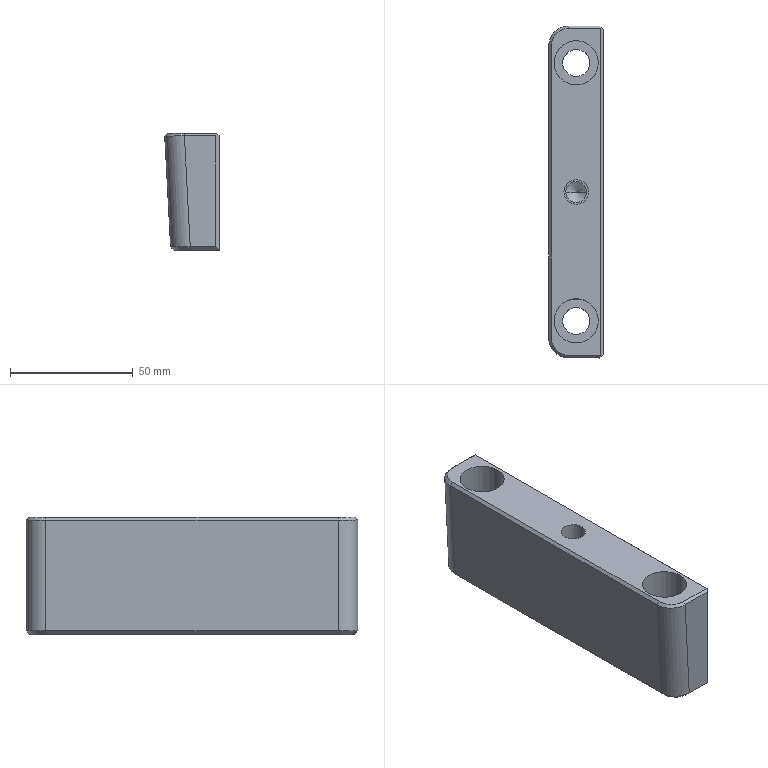Part | Creo | 1 solid | 38 faces | box 22.187 x 135.002 x 47.7 mm | volume 118010 mm3 | plane 18 | cylinder 14 | spline 4 | cone 2 | commonest cylinder face diameters 11 x4 18 x4 8.5 x2 10 x2 16 x2
STEP:
#1=CARTESIAN_POINT('',(-136.,-90.504,-72.5));
#2=VERTEX_POINT('',#1);
#3=CARTESIAN_POINT('',(-126.,-90.506,-72.5));
#4=VERTEX_POINT('',#3);
#5=CARTESIAN_POINT('',(-131.,-90.505,-72.5));
#6=DIRECTION('',(0.,0.,1.));
#7=DIRECTION('',(-1.,0.0001909,0.));
#8=AXIS2_PLACEMENT_3D('',#5,#6,#7);
#9=CIRCLE('',#8,5.);
#10=EDGE_CURVE('',#2,#4,#9,.T.);
#11=ORIENTED_EDGE('',*,*,#10,.F.);
#12=CARTESIAN_POINT('',(-131.,-90.505,-72.5));
#13=DIRECTION('',(0.,0.,1.));
#14=DIRECTION('',(1.,-0.0001909,0.));
#15=AXIS2_PLACEMENT_3D('',#12,#13,#14);
#16=CIRCLE('',#15,5.);
#17=EDGE_CURVE('',#4,#2,#16,.T.);
#18=ORIENTED_EDGE('',*,*,#17,.F.);
#19=EDGE_LOOP('',(#11,#18));
#20=FACE_OUTER_BOUND('',#19,.F.);
#21=CARTESIAN_POINT('',(-135.25,-90.504,-72.5));
#22=VERTEX_POINT('',#21);
#23=CARTESIAN_POINT('',(-126.75,-90.506,-72.5));
#24=VERTEX_POINT('',#23);
#25=CARTESIAN_POINT('',(-131.,-90.505,-72.5));
#26=DIRECTION('',(0.,0.,-1.));
#27=DIRECTION('',(-1.,0.0001909,0.));
#28=AXIS2_PLACEMENT_3D('',#25,#26,#27);
#29=CIRCLE('',#28,4.25);
#30=EDGE_CURVE('',#22,#24,#29,.T.);
#31=ORIENTED_EDGE('',*,*,#30,.F.);
#32=CARTESIAN_POINT('',(-131.,-90.505,-72.5));
#33=DIRECTION('',(0.,0.,-1.));
#34=DIRECTION('',(1.,-0.0001909,0.));
#35=AXIS2_PLACEMENT_3D('',#32,#33,#34);
#36=CIRCLE('',#35,4.25);
#37=EDGE_CURVE('',#24,#22,#36,.T.);
#38=ORIENTED_EDGE('',*,*,#37,.F.);
#39=EDGE_LOOP('',(#31,#38));
#40=FACE_BOUND('',#39,.F.);
#41=CARTESIAN_POINT('',(-131.,-90.505,-72.5));
#42=DIRECTION('',(0.,0.,-1.));
#43=DIRECTION('',(-1.,0.0001909,0.));
#44=AXIS2_PLACEMENT_3D('',#41,#42,#43);
#45=PLANE('',#44);
#46=ADVANCED_FACE('',(#20,#40),#45,.F.);
#47=CARTESIAN_POINT('',(-126.75,-90.506,-84.));
#48=VERTEX_POINT('',#47);
#49=CARTESIAN_POINT('',(-135.25,-90.504,-84.));
#50=VERTEX_POINT('',#49);
#51=CARTESIAN_POINT('',(-131.,-90.505,-84.));
#52=DIRECTION('',(0.,0.,1.));
#53=DIRECTION('',(1.,-0.0001909,0.));
#54=AXIS2_PLACEMENT_3D('',#51,#52,#53);
#55=CIRCLE('',#54,4.25);
#56=EDGE_CURVE('',#48,#50,#55,.T.);
#57=ORIENTED_EDGE('',*,*,#56,.T.);
#58=CARTESIAN_POINT('',(-135.25,-90.504,-84.));
#59=DIRECTION('',(0.,0.000000007,1.));
#60=VECTOR('',#59,11.5);
#61=LINE('',#58,#60);
#62=EDGE_CURVE('',#50,#22,#61,.T.);
#63=ORIENTED_EDGE('',*,*,#62,.T.);
#64=ORIENTED_EDGE('',*,*,#30,.T.);
#65=CARTESIAN_POINT('',(-126.75,-90.506,-84.));
#66=DIRECTION('',(0.,0.,1.));
#67=VECTOR('',#66,11.5);
#68=LINE('',#65,#67);
#69=EDGE_CURVE('',#48,#24,#68,.T.);
#70=ORIENTED_EDGE('',*,*,#69,.F.);
#71=EDGE_LOOP('',(#57,#63,#64,#70));
#72=FACE_OUTER_BOUND('',#71,.F.);
#73=CARTESIAN_POINT('',(-131.,-90.505,-87.956));
#74=DIRECTION('',(0.,0.,1.));
#75=DIRECTION('',(-1.,0.0001909,0.));
#76=AXIS2_PLACEMENT_3D('',#73,#74,#75);
#77=CYLINDRICAL_SURFACE('',#76,4.25);
#78=ADVANCED_FACE('',(#72),#77,.F.);
#79=ORIENTED_EDGE('',*,*,#56,.F.);
#80=CARTESIAN_POINT('',(-131.,-90.505,-86.554));
#81=VERTEX_POINT('',#80);
#82=CARTESIAN_POINT('',(-131.,-90.505,-86.554));
#83=DIRECTION('',(0.8572,-0.0001636,0.515));
#84=VECTOR('',#83,4.958);
#85=LINE('',#82,#84);
#86=EDGE_CURVE('',#81,#48,#85,.T.);
#87=ORIENTED_EDGE('',*,*,#86,.F.);
#88=CARTESIAN_POINT('',(-131.,-90.505,-86.554));
#89=DIRECTION('',(-0.8572,0.0001636,0.515));
#90=VECTOR('',#89,4.958);
#91=LINE('',#88,#90);
#92=EDGE_CURVE('',#81,#50,#91,.T.);
#93=ORIENTED_EDGE('',*,*,#92,.T.);
#94=EDGE_LOOP('',(#79,#87,#93));
#95=FACE_OUTER_BOUND('',#94,.F.);
#96=CARTESIAN_POINT('',(-131.,-90.505,-85.232));
#97=DIRECTION('',(0.,0.,1.));
#98=DIRECTION('',(-1.,0.0001909,0.));
#99=AXIS2_PLACEMENT_3D('',#96,#97,#98);
#100=CONICAL_SURFACE('',#99,2.2,59.);
#101=ADVANCED_FACE('',(#95),#100,.F.);
#102=CARTESIAN_POINT('',(-131.,-90.505,-84.));
#103=DIRECTION('',(0.,0.,1.));
#104=DIRECTION('',(-1.,0.0001909,0.));
#105=AXIS2_PLACEMENT_3D('',#102,#103,#104);
#106=CIRCLE('',#105,4.25);
#107=EDGE_CURVE('',#50,#48,#106,.T.);
#108=ORIENTED_EDGE('',*,*,#107,.F.);
#109=ORIENTED_EDGE('',*,*,#92,.F.);
#110=ORIENTED_EDGE('',*,*,#86,.T.);
#111=EDGE_LOOP('',(#108,#109,#110));
#112=FACE_OUTER_BOUND('',#111,.F.);
#113=CARTESIAN_POINT('',(-131.,-90.505,-85.232));
#114=DIRECTION('',(0.,0.,1.));
#115=DIRECTION('',(-1.,0.0001909,0.));
#116=AXIS2_PLACEMENT_3D('',#113,#114,#115);
#117=CONICAL_SURFACE('',#116,2.2,59.);
#118=ADVANCED_FACE('',(#112),#117,.F.);
#119=ORIENTED_EDGE('',*,*,#107,.T.);
#120=ORIENTED_EDGE('',*,*,#69,.T.);
#121=ORIENTED_EDGE('',*,*,#37,.T.);
#122=ORIENTED_EDGE('',*,*,#62,.F.);
#123=EDGE_LOOP('',(#119,#120,#121,#122));
#124=FACE_OUTER_BOUND('',#123,.F.);
#125=CARTESIAN_POINT('',(-131.,-90.505,-87.956));
#126=DIRECTION('',(0.,0.,1.));
#127=DIRECTION('',(-1.,0.0001909,0.));
#128=AXIS2_PLACEMENT_3D('',#125,#126,#127);
#129=CYLINDRICAL_SURFACE('',#128,4.25);
#130=ADVANCED_FACE('',(#124),#129,.F.);
#131=CARTESIAN_POINT('',(-126.,-90.506,-54.));
#132=VERTEX_POINT('',#131);
#133=CARTESIAN_POINT('',(-136.,-90.504,-54.));
#134=VERTEX_POINT('',#133);
#135=CARTESIAN_POINT('',(-131.,-90.505,-54.));
#136=DIRECTION('',(0.,0.,-1.));
#137=DIRECTION('',(1.,-0.0001909,0.));
#138=AXIS2_PLACEMENT_3D('',#135,#136,#137);
#139=CIRCLE('',#138,5.);
#140=EDGE_CURVE('',#132,#134,#139,.T.);
#141=ORIENTED_EDGE('',*,*,#140,.T.);
#142=CARTESIAN_POINT('',(-136.,-90.504,-54.));
#143=DIRECTION('',(0.,0.,-1.));
#144=VECTOR('',#143,18.5);
#145=LINE('',#142,#144);
#146=EDGE_CURVE('',#134,#2,#145,.T.);
#147=ORIENTED_EDGE('',*,*,#146,.T.);
#148=ORIENTED_EDGE('',*,*,#10,.T.);
#149=CARTESIAN_POINT('',(-126.,-90.506,-54.));
#150=DIRECTION('',(0.,0.,-1.));
#151=VECTOR('',#150,18.5);
#152=LINE('',#149,#151);
#153=EDGE_CURVE('',#132,#4,#152,.T.);
#154=ORIENTED_EDGE('',*,*,#153,.F.);
#155=EDGE_LOOP('',(#141,#147,#148,#154));
#156=FACE_OUTER_BOUND('',#155,.F.);
#157=CARTESIAN_POINT('',(-131.,-90.505,-45.));
#158=DIRECTION('',(0.,0.,-1.));
#159=DIRECTION('',(-1.,0.0001909,0.));
#160=AXIS2_PLACEMENT_3D('',#157,#158,#159);
#161=CYLINDRICAL_SURFACE('',#160,5.);
#162=ADVANCED_FACE('',(#156),#161,.F.);
#163=CARTESIAN_POINT('',(-120.981,-157.039,-54.));
#164=VERTEX_POINT('',#163);
#165=CARTESIAN_POINT('',(-134.055,-157.036,-54.));
#166=VERTEX_POINT('',#165);
#167=CARTESIAN_POINT('',(-120.981,-157.039,-54.));
#168=DIRECTION('',(-1.,0.0001994,0.));
#169=VECTOR('',#168,13.074);
#170=LINE('',#167,#169);
#171=EDGE_CURVE('',#164,#166,#170,.T.);
#172=ORIENTED_EDGE('',*,*,#171,.T.);
#173=CARTESIAN_POINT('',(-141.096,-150.004,-54.));
#174=VERTEX_POINT('',#173);
#175=CARTESIAN_POINT('',(-134.06,-149.999,-54.));
#176=DIRECTION('',(0.,0.,1.));
#177=DIRECTION('',(-1.,-0.0009608,0.));
#178=AXIS2_PLACEMENT_3D('',#175,#176,#177);
#179=CIRCLE('',#178,7.037);
#180=EDGE_CURVE('',#174,#166,#179,.T.);
#181=ORIENTED_EDGE('',*,*,#180,.F.);
#182=CARTESIAN_POINT('',(-141.074,-31.,-54.));
#183=VERTEX_POINT('',#182);
#184=CARTESIAN_POINT('',(-141.096,-150.004,-54.));
#185=DIRECTION('',(0.0001909,1.,0.));
#186=VECTOR('',#185,119.002);
#187=LINE('',#184,#186);
#188=EDGE_CURVE('',#174,#183,#187,.T.);
#189=ORIENTED_EDGE('',*,*,#188,.T.);
#190=CARTESIAN_POINT('',(-134.029,-23.972,-54.));
#191=VERTEX_POINT('',#190);
#192=CARTESIAN_POINT('',(-134.037,-31.009,-54.));
#193=DIRECTION('',(0.,0.,1.));
#194=DIRECTION('',(0.001347,1.,0.));
#195=AXIS2_PLACEMENT_3D('',#192,#193,#194);
#196=CIRCLE('',#195,7.037);
#197=EDGE_CURVE('',#191,#183,#196,.T.);
#198=ORIENTED_EDGE('',*,*,#197,.F.);
#199=CARTESIAN_POINT('',(-120.955,-23.975,-54.));
#200=VERTEX_POINT('',#199);
#201=CARTESIAN_POINT('',(-134.029,-23.972,-54.));
#202=DIRECTION('',(1.,-0.0001866,0.000004272));
#203=VECTOR('',#202,13.074);
#204=LINE('',#201,#203);
#205=EDGE_CURVE('',#191,#200,#204,.T.);
#206=ORIENTED_EDGE('',*,*,#205,.T.);
#207=CARTESIAN_POINT('',(-120.955,-23.975,-54.));
#208=DIRECTION('',(-0.0001909,-1.,0.));
#209=VECTOR('',#208,133.064);
#210=LINE('',#207,#209);
#211=EDGE_CURVE('',#200,#164,#210,.T.);
#212=ORIENTED_EDGE('',*,*,#211,.T.);
#213=EDGE_LOOP('',(#172,#181,#189,#198,#206,#212));
#214=FACE_OUTER_BOUND('',#213,.F.);
#215=CARTESIAN_POINT('',(-140.01,-143.003,-54.));
#216=VERTEX_POINT('',#215);
#217=CARTESIAN_POINT('',(-122.01,-143.006,-54.));
#218=VERTEX_POINT('',#217);
#219=CARTESIAN_POINT('',(-131.01,-143.005,-54.));
#220=DIRECTION('',(0.,0.,-1.));
#221=DIRECTION('',(-1.,0.0001909,0.));
#222=AXIS2_PLACEMENT_3D('',#219,#220,#221);
#223=CIRCLE('',#222,9.);
#224=EDGE_CURVE('',#216,#218,#223,.T.);
#225=ORIENTED_EDGE('',*,*,#224,.F.);
#226=CARTESIAN_POINT('',(-131.01,-143.005,-54.));
#227=DIRECTION('',(0.,0.,-1.));
#228=DIRECTION('',(1.,-0.0001909,0.));
#229=AXIS2_PLACEMENT_3D('',#226,#227,#228);
#230=CIRCLE('',#229,9.);
#231=EDGE_CURVE('',#218,#216,#230,.T.);
#232=ORIENTED_EDGE('',*,*,#231,.F.);
#233=EDGE_LOOP('',(#225,#232));
#234=FACE_BOUND('',#233,.F.);
#235=CARTESIAN_POINT('',(-131.,-90.505,-54.));
#236=DIRECTION('',(0.,0.,-1.));
#237=DIRECTION('',(-1.,0.0001909,0.));
#238=AXIS2_PLACEMENT_3D('',#235,#236,#237);
#239=CIRCLE('',#238,5.);
#240=EDGE_CURVE('',#134,#132,#239,.T.);
#241=ORIENTED_EDGE('',*,*,#240,.F.);
#242=ORIENTED_EDGE('',*,*,#140,.F.);
#243=EDGE_LOOP('',(#241,#242));
#244=FACE_BOUND('',#243,.F.);
#245=CARTESIAN_POINT('',(-139.99,-38.003,-54.));
#246=VERTEX_POINT('',#245);
#247=CARTESIAN_POINT('',(-121.99,-38.006,-54.));
#248=VERTEX_POINT('',#247);
#249=CARTESIAN_POINT('',(-130.99,-38.005,-54.));
#250=DIRECTION('',(0.,0.,-1.));
#251=DIRECTION('',(-1.,0.0001909,0.));
#252=AXIS2_PLACEMENT_3D('',#249,#250,#251);
#253=CIRCLE('',#252,9.);
#254=EDGE_CURVE('',#246,#248,#253,.T.);
#255=ORIENTED_EDGE('',*,*,#254,.F.);
#256=CARTESIAN_POINT('',(-130.99,-38.005,-54.));
#257=DIRECTION('',(0.,0.,-1.));
#258=DIRECTION('',(1.,-0.0001909,0.));
#259=AXIS2_PLACEMENT_3D('',#256,#257,#258);
#260=CIRCLE('',#259,9.);
#261=EDGE_CURVE('',#248,#246,#260,.T.);
#262=ORIENTED_EDGE('',*,*,#261,.F.);
#263=EDGE_LOOP('',(#255,#262));
#264=FACE_BOUND('',#263,.F.);
#265=CARTESIAN_POINT('',(-249.985,-12.982,-54.));
#266=DIRECTION('',(0.,0.,-1.));
#267=DIRECTION('',(-0.0001909,-1.,0.));
#268=AXIS2_PLACEMENT_3D('',#265,#266,#267);
#269=PLANE('',#268);
#270=ADVANCED_FACE('',(#214,#234,#244,#264),#269,.F.);
#271=CARTESIAN_POINT('',(-134.056,-158.004,-54.968));
#272=VERTEX_POINT('',#271);
#273=CARTESIAN_POINT('',(-121.436,-158.007,-54.968));
#274=VERTEX_POINT('',#273);
#275=CARTESIAN_POINT('',(-134.056,-158.004,-54.968));
#276=DIRECTION('',(1.,-0.0001948,0.000003922));
#277=VECTOR('',#276,12.62);
#278=LINE('',#275,#277);
#279=EDGE_CURVE('',#272,#274,#278,.T.);
#280=ORIENTED_EDGE('',*,*,#279,.F.);
#281=CARTESIAN_POINT('',(-134.056,-158.004,-54.968));
#282=DIRECTION('',(0.0008599,0.7071,0.7071));
#283=VECTOR('',#282,1.369);
#284=LINE('',#281,#283);
#285=EDGE_CURVE('',#272,#166,#284,.T.);
#286=ORIENTED_EDGE('',*,*,#285,.T.);
#287=ORIENTED_EDGE('',*,*,#171,.F.);
#288=CARTESIAN_POINT('',(-120.724,-157.295,-54.256));
#289=VERTEX_POINT('',#288);
#290=CARTESIAN_POINT('',(-120.724,-157.295,-54.256));
#291=DIRECTION('',(-0.5772,0.5775,0.5774));
#292=VECTOR('',#291,0.444);
#293=LINE('',#290,#292);
#294=EDGE_CURVE('',#289,#164,#293,.T.);
#295=ORIENTED_EDGE('',*,*,#294,.F.);
#296=CARTESIAN_POINT('',(-121.436,-158.007,-54.968));
#297=DIRECTION('',(0.5775,0.5772,0.5774));
#298=VECTOR('',#297,1.233);
#299=LINE('',#296,#298);
#300=EDGE_CURVE('',#274,#289,#299,.T.);
#301=ORIENTED_EDGE('',*,*,#300,.F.);
#302=EDGE_LOOP('',(#280,#286,#287,#295,#301));
#303=FACE_OUTER_BOUND('',#302,.F.);
#304=CARTESIAN_POINT('',(-120.013,-158.007,-54.968));
#305=DIRECTION('',(0.000135,0.7071,-0.7071));
#306=DIRECTION('',(-1.,0.0001909,0.));
#307=AXIS2_PLACEMENT_3D('',#304,#305,#306);
#308=PLANE('',#307);
#309=ADVANCED_FACE('',(#303),#308,.F.);
#310=CARTESIAN_POINT('',(-121.436,-158.007,-100.119));
#311=VERTEX_POINT('',#310);
#312=CARTESIAN_POINT('',(-121.436,-158.007,-54.968));
#313=DIRECTION('',(0.,0.,-1.));
#314=VECTOR('',#313,45.151);
#315=LINE('',#312,#314);
#316=EDGE_CURVE('',#274,#311,#315,.T.);
#317=ORIENTED_EDGE('',*,*,#316,.T.);
#318=CARTESIAN_POINT('',(-131.821,-158.005,-100.119));
#319=VERTEX_POINT('',#318);
#320=CARTESIAN_POINT('',(-121.436,-158.007,-100.119));
#321=DIRECTION('',(-1.,0.0001909,-0.00001405));
#322=VECTOR('',#321,10.384);
#323=LINE('',#320,#322);
#324=EDGE_CURVE('',#311,#319,#323,.T.);
#325=ORIENTED_EDGE('',*,*,#324,.T.);
#326=CARTESIAN_POINT('',(-134.187,-158.004,-54.97));
#327=VERTEX_POINT('',#326);
#328=CARTESIAN_POINT('',(-134.187,-158.004,-54.97));
#329=DIRECTION('',(0.05234,-0.00001101,-0.9986));
#330=VECTOR('',#329,45.211);
#331=LINE('',#328,#330);
#332=EDGE_CURVE('',#327,#319,#331,.T.);
#333=ORIENTED_EDGE('',*,*,#332,.F.);
#334=CARTESIAN_POINT('',(-134.056,-158.004,-54.968));
#335=CARTESIAN_POINT('',(-134.071,-158.004,-54.968));
#336=CARTESIAN_POINT('',(-134.1,-158.004,-54.968));
#337=CARTESIAN_POINT('',(-134.143,-158.004,-54.969));
#338=CARTESIAN_POINT('',(-134.172,-158.004,-54.97));
#339=B_SPLINE_CURVE_WITH_KNOTS('',3,(#334,#335,#336,#337,#338,#326),.UNSPECIFIED.,.F.,.F.,(4,1,1,4),(0.,0.3333,0.6667,1.),.UNSPECIFIED.);
#340=EDGE_CURVE('',#272,#327,#339,.T.);
#341=ORIENTED_EDGE('',*,*,#340,.F.);
#342=ORIENTED_EDGE('',*,*,#279,.T.);
#343=EDGE_LOOP('',(#317,#325,#333,#341,#342));
#344=FACE_OUTER_BOUND('',#343,.F.);
#345=CARTESIAN_POINT('',(-120.013,-158.007,-66.5));
#346=DIRECTION('',(0.0001909,1.,0.));
#347=DIRECTION('',(-1.,0.0001909,0.));
#348=AXIS2_PLACEMENT_3D('',#345,#346,#347);
#349=PLANE('',#348);
#350=ADVANCED_FACE('',(#344),#349,.F.);
#351=CARTESIAN_POINT('',(-120.,-156.571,-54.981));
#352=VERTEX_POINT('',#351);
#353=CARTESIAN_POINT('',(-120.,-156.571,-101.555));
#354=VERTEX_POINT('',#353);
#355=CARTESIAN_POINT('',(-120.,-156.571,-54.981));
#356=DIRECTION('',(0.,0.,-1.));
#357=VECTOR('',#356,46.575);
#358=LINE('',#355,#357);
#359=EDGE_CURVE('',#352,#354,#358,.T.);
#360=ORIENTED_EDGE('',*,*,#359,.T.);
#361=CARTESIAN_POINT('',(-121.436,-158.007,-100.119));
#362=DIRECTION('',(0.5775,0.5772,-0.5774));
#363=VECTOR('',#362,2.487);
#364=LINE('',#361,#363);
#365=EDGE_CURVE('',#311,#354,#364,.T.);
#366=ORIENTED_EDGE('',*,*,#365,.F.);
#367=ORIENTED_EDGE('',*,*,#316,.F.);
#368=ORIENTED_EDGE('',*,*,#300,.T.);
#369=CARTESIAN_POINT('',(-120.724,-157.295,-54.256));
#370=DIRECTION('',(0.5775,0.5772,-0.5774));
#371=VECTOR('',#370,1.255);
#372=LINE('',#369,#371);
#373=EDGE_CURVE('',#289,#352,#372,.T.);
#374=ORIENTED_EDGE('',*,*,#373,.T.);
#375=EDGE_LOOP('',(#360,#366,#367,#368,#374));
#376=FACE_OUTER_BOUND('',#375,.F.);
#377=CARTESIAN_POINT('',(-120.724,-157.295,-79.31));
#378=DIRECTION('',(0.707,-0.7072,0.));
#379=DIRECTION('',(0.7072,0.707,0.));
#380=AXIS2_PLACEMENT_3D('',#377,#378,#379);
#381=PLANE('',#380);
#382=ADVANCED_FACE('',(#376),#381,.T.);
#383=CARTESIAN_POINT('',(-120.,-24.418,-101.53));
#384=VERTEX_POINT('',#383);
#385=CARTESIAN_POINT('',(-120.,-24.418,-54.955));
#386=VERTEX_POINT('',#385);
#387=CARTESIAN_POINT('',(-120.,-24.418,-101.53));
#388=DIRECTION('',(0.,0.000000001,1.));
#389=VECTOR('',#388,46.575);
#390=LINE('',#387,#389);
#391=EDGE_CURVE('',#384,#386,#390,.T.);
#392=ORIENTED_EDGE('',*,*,#391,.F.);
#393=CARTESIAN_POINT('',(-120.,-24.587,-101.7));
#394=VERTEX_POINT('',#393);
#395=CARTESIAN_POINT('',(-120.,-24.587,-101.7));
#396=DIRECTION('',(0.000000042,0.7071,0.7071));
#397=VECTOR('',#396,0.2402);
#398=LINE('',#395,#397);
#399=EDGE_CURVE('',#394,#384,#398,.T.);
#400=ORIENTED_EDGE('',*,*,#399,.F.);
#401=CARTESIAN_POINT('',(-120.,-156.426,-101.7));
#402=VERTEX_POINT('',#401);
#403=CARTESIAN_POINT('',(-120.,-24.587,-101.7));
#404=DIRECTION('',(-0.000000059,-1.,0.));
#405=VECTOR('',#404,131.839);
#406=LINE('',#403,#405);
#407=EDGE_CURVE('',#394,#402,#406,.T.);
#408=ORIENTED_EDGE('',*,*,#407,.T.);
#409=CARTESIAN_POINT('',(-120.,-156.571,-101.555));
#410=DIRECTION('',(0.000000042,0.7071,-0.7071));
#411=VECTOR('',#410,0.2045);
#412=LINE('',#409,#411);
#413=EDGE_CURVE('',#354,#402,#412,.T.);
#414=ORIENTED_EDGE('',*,*,#413,.F.);
#415=ORIENTED_EDGE('',*,*,#359,.F.);
#416=CARTESIAN_POINT('',(-120.,-156.571,-54.981));
#417=DIRECTION('',(0.000000059,1.,0.0001908));
#418=VECTOR('',#417,132.153);
#419=LINE('',#416,#418);
#420=EDGE_CURVE('',#352,#386,#419,.T.);
#421=ORIENTED_EDGE('',*,*,#420,.T.);
#422=EDGE_LOOP('',(#392,#400,#408,#414,#415,#421));
#423=FACE_OUTER_BOUND('',#422,.F.);
#424=CARTESIAN_POINT('',(-120.,0.000007043,105.3));
#425=DIRECTION('',(-1.,0.000000059,0.));
#426=DIRECTION('',(-0.000000059,-1.,0.));
#427=AXIS2_PLACEMENT_3D('',#424,#425,#426);
#428=PLANE('',#427);
#429=ADVANCED_FACE('',(#423),#428,.F.);
#430=CARTESIAN_POINT('',(-120.699,-23.718,-54.256));
#431=VERTEX_POINT('',#430);
#432=CARTESIAN_POINT('',(-121.411,-23.007,-54.968));
#433=VERTEX_POINT('',#432);
#434=CARTESIAN_POINT('',(-120.699,-23.718,-54.256));
#435=DIRECTION('',(-0.5772,0.5775,-0.5774));
#436=VECTOR('',#435,1.233);
#437=LINE('',#434,#436);
#438=EDGE_CURVE('',#431,#433,#437,.T.);
#439=ORIENTED_EDGE('',*,*,#438,.T.);
#440=CARTESIAN_POINT('',(-121.411,-23.007,-100.119));
#441=VERTEX_POINT('',#440);
#442=CARTESIAN_POINT('',(-121.411,-23.007,-100.119));
#443=DIRECTION('',(0.,0.,1.));
#444=VECTOR('',#443,45.151);
#445=LINE('',#442,#444);
#446=EDGE_CURVE('',#441,#433,#445,.T.);
#447=ORIENTED_EDGE('',*,*,#446,.F.);
#448=CARTESIAN_POINT('',(-120.,-24.418,-101.53));
#449=DIRECTION('',(-0.5772,0.5775,0.5774));
#450=VECTOR('',#449,2.444);
#451=LINE('',#448,#450);
#452=EDGE_CURVE('',#384,#441,#451,.T.);
#453=ORIENTED_EDGE('',*,*,#452,.F.);
#454=ORIENTED_EDGE('',*,*,#391,.T.);
#455=CARTESIAN_POINT('',(-120.,-24.418,-54.955));
#456=DIRECTION('',(-0.5772,0.5775,0.5774));
#457=VECTOR('',#456,1.211);
#458=LINE('',#455,#457);
#459=EDGE_CURVE('',#386,#431,#458,.T.);
#460=ORIENTED_EDGE('',*,*,#459,.T.);
#461=EDGE_LOOP('',(#439,#447,#453,#454,#460));
#462=FACE_OUTER_BOUND('',#461,.F.);
#463=CARTESIAN_POINT('',(-120.699,-23.718,-79.31));
#464=DIRECTION('',(0.7072,0.707,0.));
#465=DIRECTION('',(0.707,-0.7072,0.));
#466=AXIS2_PLACEMENT_3D('',#463,#464,#465);
#467=PLANE('',#466);
#468=ADVANCED_FACE('',(#462),#467,.T.);
#469=CARTESIAN_POINT('',(-134.03,-23.004,-54.968));
#470=VERTEX_POINT('',#469);
#471=CARTESIAN_POINT('',(-134.029,-23.972,-54.));
#472=DIRECTION('',(-0.0005901,0.7071,-0.7071));
#473=VECTOR('',#472,1.369);
#474=LINE('',#471,#473);
#475=EDGE_CURVE('',#191,#470,#474,.T.);
#476=ORIENTED_EDGE('',*,*,#475,.T.);
#477=CARTESIAN_POINT('',(-121.411,-23.007,-54.968));
#478=DIRECTION('',(-1.,0.000187,-0.000003922));
#479=VECTOR('',#478,12.62);
#480=LINE('',#477,#479);
#481=EDGE_CURVE('',#433,#470,#480,.T.);
#482=ORIENTED_EDGE('',*,*,#481,.F.);
#483=ORIENTED_EDGE('',*,*,#438,.F.);
#484=CARTESIAN_POINT('',(-120.955,-23.975,-54.));
#485=DIRECTION('',(0.5775,0.5772,-0.5774));
#486=VECTOR('',#485,0.444);
#487=LINE('',#484,#486);
#488=EDGE_CURVE('',#200,#431,#487,.T.);
#489=ORIENTED_EDGE('',*,*,#488,.F.);
#490=ORIENTED_EDGE('',*,*,#205,.F.);
#491=EDGE_LOOP('',(#476,#482,#483,#489,#490));
#492=FACE_OUTER_BOUND('',#491,.F.);
#493=CARTESIAN_POINT('',(-249.987,-23.95,-54.));
#494=DIRECTION('',(0.000135,0.7071,0.7071));
#495=DIRECTION('',(1.,-0.0001909,0.));
#496=AXIS2_PLACEMENT_3D('',#493,#494,#495);
#497=PLANE('',#496);
#498=ADVANCED_FACE('',(#492),#497,.T.);
#499=CARTESIAN_POINT('',(-142.164,-31.003,-55.15));
#500=VERTEX_POINT('',#499);
#501=CARTESIAN_POINT('',(-142.164,-31.003,-55.15));
#502=DIRECTION('',(0.6883,0.0004876,0.7254));
#503=VECTOR('',#502,1.585);
#504=LINE('',#501,#503);
#505=EDGE_CURVE('',#500,#183,#504,.T.);
#506=ORIENTED_EDGE('',*,*,#505,.F.);
#507=CARTESIAN_POINT('',(-134.161,-23.004,-54.97));
#508=VERTEX_POINT('',#507);
#509=CARTESIAN_POINT('',(-134.161,-23.004,-54.97));
#510=CARTESIAN_POINT('',(-134.684,-23.004,-54.982));
#511=CARTESIAN_POINT('',(-135.73,-23.107,-55.005));
#512=CARTESIAN_POINT('',(-137.24,-23.564,-55.039));
#513=CARTESIAN_POINT('',(-138.632,-24.307,-55.071));
#514=CARTESIAN_POINT('',(-139.853,-25.307,-55.098));
#515=CARTESIAN_POINT('',(-140.856,-26.527,-55.121));
#516=CARTESIAN_POINT('',(-141.601,-27.919,-55.137));
#517=CARTESIAN_POINT('',(-142.061,-29.431,-55.147));
#518=CARTESIAN_POINT('',(-142.164,-30.479,-55.15));
#519=CARTESIAN_POINT('',(-142.164,-31.003,-55.15));
#520=B_SPLINE_CURVE_WITH_KNOTS('',3,(#509,#510,#511,#512,#513,#514,#515,#516,#517,#518,#519),.UNSPECIFIED.,.F.,.F.,(4,1,1,1,1,1,1,1,4),(0.,0.125,0.25,0.375,0.5,0.625,0.75,0.875,1.),.UNSPECIFIED.);
#521=EDGE_CURVE('',#508,#500,#520,.T.);
#522=ORIENTED_EDGE('',*,*,#521,.F.);
#523=CARTESIAN_POINT('',(-134.045,-23.004,-54.968));
#524=CARTESIAN_POINT('',(-134.074,-23.004,-54.969));
#525=CARTESIAN_POINT('',(-134.118,-23.004,-54.968));
#526=CARTESIAN_POINT('',(-134.147,-23.004,-54.97));
#527=CARTESIAN_POINT('',(-134.161,-23.004,-54.97));
#528=B_SPLINE_CURVE_WITH_KNOTS('',3,(#469,#523,#524,#525,#526,#527),.UNSPECIFIED.,.F.,.F.,(4,1,1,4),(0.,0.3333,0.6667,1.),.UNSPECIFIED.);
#529=EDGE_CURVE('',#470,#508,#528,.T.);
#530=ORIENTED_EDGE('',*,*,#529,.F.);
#531=ORIENTED_EDGE('',*,*,#475,.F.);
#532=ORIENTED_EDGE('',*,*,#197,.T.);
#533=EDGE_LOOP('',(#506,#522,#530,#531,#532));
#534=FACE_OUTER_BOUND('',#533,.F.);
#535=CARTESIAN_POINT('',(-142.284,-31.262,-55.279));
#536=CARTESIAN_POINT('',(-141.838,-31.248,-54.81));
#537=CARTESIAN_POINT('',(-141.393,-31.234,-54.34));
#538=CARTESIAN_POINT('',(-140.947,-31.22,-53.87));
#539=CARTESIAN_POINT('',(-142.286,-31.175,-55.279));
#540=CARTESIAN_POINT('',(-141.841,-31.166,-54.81));
#541=CARTESIAN_POINT('',(-141.395,-31.157,-54.34));
#542=CARTESIAN_POINT('',(-140.949,-31.148,-53.87));
#543=CARTESIAN_POINT('',(-142.321,-28.928,-55.28));
#544=CARTESIAN_POINT('',(-141.873,-29.041,-54.81));
#545=CARTESIAN_POINT('',(-141.426,-29.153,-54.34));
#546=CARTESIAN_POINT('',(-140.978,-29.265,-53.87));
#547=CARTESIAN_POINT('',(-140.496,-24.54,-55.266));
#548=CARTESIAN_POINT('',(-140.146,-24.889,-54.801));
#549=CARTESIAN_POINT('',(-139.797,-25.239,-54.336));
#550=CARTESIAN_POINT('',(-139.447,-25.589,-53.871));
#551=CARTESIAN_POINT('',(-136.104,-22.72,-55.232));
#552=CARTESIAN_POINT('',(-135.992,-23.169,-54.779));
#553=CARTESIAN_POINT('',(-135.88,-23.617,-54.327));
#554=CARTESIAN_POINT('',(-135.768,-24.065,-53.875));
#555=CARTESIAN_POINT('',(-133.857,-22.758,-55.214));
#556=CARTESIAN_POINT('',(-133.867,-23.205,-54.768));
#557=CARTESIAN_POINT('',(-133.876,-23.651,-54.322));
#558=CARTESIAN_POINT('',(-133.886,-24.097,-53.877));
#559=CARTESIAN_POINT('',(-133.771,-22.761,-55.214));
#560=CARTESIAN_POINT('',(-133.785,-23.207,-54.768));
#561=CARTESIAN_POINT('',(-133.799,-23.654,-54.322));
#562=CARTESIAN_POINT('',(-133.813,-24.1,-53.877));
#563=B_SPLINE_SURFACE_WITH_KNOTS('',3,3,((#535,#536,#537,#538),(#539,#540,#541,#542),(#543,#544,#545,#546),(#547,#548,#549,#550),(#551,#552,#553,#554),(#555,#556,#557,#558),(#559,#560,#561,#562)),.UNSPECIFIED.,.F.,.F.,.F.,(4,1,1,1,4),(4,4),(-0.02,0.,0.5,1.,1.02),(0.1697,1.084),.UNSPECIFIED.);
#564=ADVANCED_FACE('',(#534),#563,.F.);
#565=ORIENTED_EDGE('',*,*,#505,.T.);
#566=ORIENTED_EDGE('',*,*,#188,.F.);
#567=CARTESIAN_POINT('',(-142.187,-150.003,-55.15));
#568=VERTEX_POINT('',#567);
#569=CARTESIAN_POINT('',(-141.096,-150.004,-54.));
#570=DIRECTION('',(-0.6883,0.0007499,-0.7254));
#571=VECTOR('',#570,1.585);
#572=LINE('',#569,#571);
#573=EDGE_CURVE('',#174,#568,#572,.T.);
#574=ORIENTED_EDGE('',*,*,#573,.T.);
#575=CARTESIAN_POINT('',(-142.164,-31.003,-55.15));
#576=DIRECTION('',(-0.0001909,-1.,0.));
#577=VECTOR('',#576,119.);
#578=LINE('',#575,#577);
#579=EDGE_CURVE('',#500,#568,#578,.T.);
#580=ORIENTED_EDGE('',*,*,#579,.F.);
#581=EDGE_LOOP('',(#565,#566,#574,#580));
#582=FACE_OUTER_BOUND('',#581,.F.);
#583=CARTESIAN_POINT('',(-141.07,-13.003,-54.));
#584=DIRECTION('',(-0.7254,0.0001385,0.6884));
#585=DIRECTION('',(0.0001909,1.,0.));
#586=AXIS2_PLACEMENT_3D('',#583,#584,#585);
#587=PLANE('',#586);
#588=ADVANCED_FACE('',(#582),#587,.T.);
#589=ORIENTED_EDGE('',*,*,#573,.F.);
#590=ORIENTED_EDGE('',*,*,#180,.T.);
#591=ORIENTED_EDGE('',*,*,#285,.F.);
#592=ORIENTED_EDGE('',*,*,#340,.T.);
#593=CARTESIAN_POINT('',(-142.187,-150.527,-55.15));
#594=CARTESIAN_POINT('',(-142.084,-151.575,-55.147));
#595=CARTESIAN_POINT('',(-141.625,-153.086,-55.137));
#596=CARTESIAN_POINT('',(-140.88,-154.479,-55.121));
#597=CARTESIAN_POINT('',(-139.878,-155.699,-55.098));
#598=CARTESIAN_POINT('',(-138.658,-156.7,-55.071));
#599=CARTESIAN_POINT('',(-137.266,-157.443,-55.039));
#600=CARTESIAN_POINT('',(-135.756,-157.901,-55.005));
#601=CARTESIAN_POINT('',(-134.71,-158.004,-54.982));
#602=CARTESIAN_POINT('',(-134.187,-158.004,-54.97));
#603=B_SPLINE_CURVE_WITH_KNOTS('',3,(#567,#593,#594,#595,#596,#597,#598,#599,#600,#601,#602),.UNSPECIFIED.,.F.,.F.,(4,1,1,1,1,1,1,1,4),(0.,0.125,0.25,0.375,0.5,0.625,0.75,0.875,1.),.UNSPECIFIED.);
#604=EDGE_CURVE('',#568,#327,#603,.T.);
#605=ORIENTED_EDGE('',*,*,#604,.F.);
#606=EDGE_LOOP('',(#589,#590,#591,#592,#605));
#607=FACE_OUTER_BOUND('',#606,.F.);
#608=CARTESIAN_POINT('',(-133.797,-158.247,-55.214));
#609=CARTESIAN_POINT('',(-133.811,-157.801,-54.768));
#610=CARTESIAN_POINT('',(-133.825,-157.355,-54.322));
#611=CARTESIAN_POINT('',(-133.839,-156.909,-53.877));
#612=CARTESIAN_POINT('',(-133.883,-158.25,-55.214));
#613=CARTESIAN_POINT('',(-133.892,-157.804,-54.768));
#614=CARTESIAN_POINT('',(-133.902,-157.357,-54.322));
#615=CARTESIAN_POINT('',(-133.911,-156.911,-53.877));
#616=CARTESIAN_POINT('',(-136.13,-158.287,-55.232));
#617=CARTESIAN_POINT('',(-136.018,-157.839,-54.779));
#618=CARTESIAN_POINT('',(-135.906,-157.391,-54.327));
#619=CARTESIAN_POINT('',(-135.793,-156.942,-53.875));
#620=CARTESIAN_POINT('',(-140.521,-156.466,-55.266));
#621=CARTESIAN_POINT('',(-140.171,-156.117,-54.801));
#622=CARTESIAN_POINT('',(-139.822,-155.767,-54.336));
#623=CARTESIAN_POINT('',(-139.472,-155.418,-53.871));
#624=CARTESIAN_POINT('',(-142.345,-152.077,-55.28));
#625=CARTESIAN_POINT('',(-141.897,-151.965,-54.81));
#626=CARTESIAN_POINT('',(-141.449,-151.852,-54.34));
#627=CARTESIAN_POINT('',(-141.001,-151.74,-53.87));
#628=CARTESIAN_POINT('',(-142.309,-149.83,-55.279));
#629=CARTESIAN_POINT('',(-141.863,-149.839,-54.81));
#630=CARTESIAN_POINT('',(-141.418,-149.849,-54.34));
#631=CARTESIAN_POINT('',(-140.972,-149.858,-53.87));
#632=CARTESIAN_POINT('',(-142.306,-149.743,-55.279));
#633=CARTESIAN_POINT('',(-141.861,-149.757,-54.81));
#634=CARTESIAN_POINT('',(-141.415,-149.772,-54.34));
#635=CARTESIAN_POINT('',(-140.97,-149.786,-53.87));
#636=B_SPLINE_SURFACE_WITH_KNOTS('',3,3,((#608,#609,#610,#611),(#612,#613,#614,#615),(#616,#617,#618,#619),(#620,#621,#622,#623),(#624,#625,#626,#627),(#628,#629,#630,#631),(#632,#633,#634,#635)),.UNSPECIFIED.,.F.,.F.,.F.,(4,1,1,1,4),(4,4),(-0.02,0.,0.5,1.,1.02),(0.1697,1.084),.UNSPECIFIED.);
#637=ADVANCED_FACE('',(#607),#636,.F.);
#638=ORIENTED_EDGE('',*,*,#332,.T.);
#639=CARTESIAN_POINT('',(-139.826,-150.003,-100.202));
#640=VERTEX_POINT('',#639);
#641=CARTESIAN_POINT('',(-139.826,-150.003,-100.202));
#642=CARTESIAN_POINT('',(-139.826,-150.526,-100.201));
#643=CARTESIAN_POINT('',(-139.723,-151.573,-100.202));
#644=CARTESIAN_POINT('',(-139.265,-153.083,-100.196));
#645=CARTESIAN_POINT('',(-138.521,-154.475,-100.189));
#646=CARTESIAN_POINT('',(-137.519,-155.696,-100.178));
#647=CARTESIAN_POINT('',(-136.299,-156.697,-100.166));
#648=CARTESIAN_POINT('',(-134.906,-157.442,-100.151));
#649=CARTESIAN_POINT('',(-133.394,-157.901,-100.136));
#650=CARTESIAN_POINT('',(-132.345,-158.004,-100.125));
#651=CARTESIAN_POINT('',(-131.821,-158.005,-100.119));
#652=B_SPLINE_CURVE_WITH_KNOTS('',3,(#641,#642,#643,#644,#645,#646,#647,#648,#649,#650,#651),.UNSPECIFIED.,.F.,.F.,(4,1,1,1,1,1,1,1,4),(0.,0.125,0.25,0.375,0.5,0.625,0.75,0.875,1.),.UNSPECIFIED.);
#653=EDGE_CURVE('',#640,#319,#652,.T.);
#654=ORIENTED_EDGE('',*,*,#653,.F.);
#655=CARTESIAN_POINT('',(-142.187,-150.003,-55.15));
#656=DIRECTION('',(0.05234,-0.000009988,-0.9986));
#657=VECTOR('',#656,45.114);
#658=LINE('',#655,#657);
#659=EDGE_CURVE('',#568,#640,#658,.T.);
#660=ORIENTED_EDGE('',*,*,#659,.F.);
#661=ORIENTED_EDGE('',*,*,#604,.T.);
#662=EDGE_LOOP('',(#638,#654,#660,#661));
#663=FACE_OUTER_BOUND('',#662,.F.);
#664=CARTESIAN_POINT('',(-136.952,-150.004,-2.184));
#665=DIRECTION('',(0.05234,-0.00000999,-0.9986));
#666=DIRECTION('',(-0.0001909,-1.,0.));
#667=AXIS2_PLACEMENT_3D('',#664,#665,#666);
#668=CYLINDRICAL_SURFACE('',#667,8.);
#669=ADVANCED_FACE('',(#663),#668,.T.);
#670=CARTESIAN_POINT('',(-138.247,-150.004,-101.7));
#671=VERTEX_POINT('',#670);
#672=CARTESIAN_POINT('',(-138.247,-150.004,-101.7));
#673=DIRECTION('',(-0.7254,0.0004399,0.6883));
#674=VECTOR('',#673,2.176);
#675=LINE('',#672,#674);
#676=EDGE_CURVE('',#671,#640,#675,.T.);
#677=ORIENTED_EDGE('',*,*,#676,.T.);
#678=ORIENTED_EDGE('',*,*,#653,.T.);
#679=CARTESIAN_POINT('',(-131.821,-156.424,-101.7));
#680=VERTEX_POINT('',#679);
#681=CARTESIAN_POINT('',(-131.821,-156.424,-101.7));
#682=DIRECTION('',(0.0001779,-0.7071,0.7071));
#683=VECTOR('',#682,2.235);
#684=LINE('',#681,#683);
#685=EDGE_CURVE('',#680,#319,#684,.T.);
#686=ORIENTED_EDGE('',*,*,#685,.F.);
#687=CARTESIAN_POINT('',(-132.189,-156.424,-101.7));
#688=CARTESIAN_POINT('',(-132.99,-156.355,-101.7));
#689=CARTESIAN_POINT('',(-134.193,-156.018,-101.7));
#690=CARTESIAN_POINT('',(-135.366,-155.412,-101.7));
#691=CARTESIAN_POINT('',(-136.393,-154.579,-101.7));
#692=CARTESIAN_POINT('',(-137.229,-153.554,-101.7));
#693=CARTESIAN_POINT('',(-137.837,-152.384,-101.7));
#694=CARTESIAN_POINT('',(-138.178,-151.179,-101.7));
#695=CARTESIAN_POINT('',(-138.246,-150.376,-101.7));
#696=CARTESIAN_POINT('',(-138.247,-150.004,-101.7));
#697=B_SPLINE_CURVE_WITH_KNOTS('',3,(#679,#687,#688,#689,#690,#691,#692,#693,#694,#695,#696),.UNSPECIFIED.,.F.,.F.,(4,1,1,1,1,1,1,1,4),(0.,0.1103,0.24,0.3696,0.4992,0.6289,0.7585,0.8881,1.),.UNSPECIFIED.);
#698=EDGE_CURVE('',#680,#671,#697,.T.);
#699=ORIENTED_EDGE('',*,*,#698,.T.);
#700=EDGE_LOOP('',(#677,#678,#686,#699));
#701=FACE_OUTER_BOUND('',#700,.F.);
#702=CARTESIAN_POINT('',(-139.953,-149.875,-100.082));
#703=CARTESIAN_POINT('',(-139.342,-149.885,-100.661));
#704=CARTESIAN_POINT('',(-138.731,-149.895,-101.241));
#705=CARTESIAN_POINT('',(-138.121,-149.904,-101.82));
#706=CARTESIAN_POINT('',(-139.953,-149.918,-100.082));
#707=CARTESIAN_POINT('',(-139.342,-149.924,-100.661));
#708=CARTESIAN_POINT('',(-138.731,-149.931,-101.241));
#709=CARTESIAN_POINT('',(-138.121,-149.937,-101.82));
#710=CARTESIAN_POINT('',(-139.955,-150.431,-100.082));
#711=CARTESIAN_POINT('',(-139.344,-150.399,-100.661));
#712=CARTESIAN_POINT('',(-138.733,-150.367,-101.241));
#713=CARTESIAN_POINT('',(-138.123,-150.334,-101.82));
#714=CARTESIAN_POINT('',(-139.865,-151.492,-100.081));
#715=CARTESIAN_POINT('',(-139.261,-151.38,-100.661));
#716=CARTESIAN_POINT('',(-138.657,-151.268,-101.241));
#717=CARTESIAN_POINT('',(-138.053,-151.156,-101.82));
#718=CARTESIAN_POINT('',(-139.434,-153.017,-100.076));
#719=CARTESIAN_POINT('',(-138.862,-152.79,-100.658));
#720=CARTESIAN_POINT('',(-138.29,-152.563,-101.239));
#721=CARTESIAN_POINT('',(-137.719,-152.337,-101.821));
#722=CARTESIAN_POINT('',(-138.664,-154.498,-100.068));
#723=CARTESIAN_POINT('',(-138.15,-154.16,-100.652));
#724=CARTESIAN_POINT('',(-137.636,-153.822,-101.237));
#725=CARTESIAN_POINT('',(-137.122,-153.484,-101.821));
#726=CARTESIAN_POINT('',(-137.607,-155.795,-100.056));
#727=CARTESIAN_POINT('',(-137.172,-155.36,-100.645));
#728=CARTESIAN_POINT('',(-136.738,-154.924,-101.234));
#729=CARTESIAN_POINT('',(-136.303,-154.488,-101.822));
#730=CARTESIAN_POINT('',(-136.307,-156.85,-100.042));
#731=CARTESIAN_POINT('',(-135.97,-156.335,-100.636));
#732=CARTESIAN_POINT('',(-135.633,-155.82,-101.229));
#733=CARTESIAN_POINT('',(-135.296,-155.305,-101.823));
#734=CARTESIAN_POINT('',(-134.822,-157.618,-100.025));
#735=CARTESIAN_POINT('',(-134.597,-157.045,-100.625));
#736=CARTESIAN_POINT('',(-134.372,-156.472,-101.225));
#737=CARTESIAN_POINT('',(-134.146,-155.899,-101.825));
#738=CARTESIAN_POINT('',(-133.301,-158.044,-100.009));
#739=CARTESIAN_POINT('',(-133.189,-157.439,-100.614));
#740=CARTESIAN_POINT('',(-133.078,-156.834,-101.22));
#741=CARTESIAN_POINT('',(-132.967,-156.229,-101.826));
#742=CARTESIAN_POINT('',(-132.243,-158.136,-99.997));
#743=CARTESIAN_POINT('',(-132.211,-157.524,-100.607));
#744=CARTESIAN_POINT('',(-132.18,-156.912,-101.217));
#745=CARTESIAN_POINT('',(-132.148,-156.3,-101.827));
#746=CARTESIAN_POINT('',(-131.736,-158.131,-99.992));
#747=CARTESIAN_POINT('',(-131.742,-157.52,-100.603));
#748=CARTESIAN_POINT('',(-131.748,-156.908,-101.215));
#749=CARTESIAN_POINT('',(-131.754,-156.297,-101.827));
#750=CARTESIAN_POINT('',(-131.693,-158.131,-99.991));
#751=CARTESIAN_POINT('',(-131.703,-157.519,-100.603));
#752=CARTESIAN_POINT('',(-131.712,-156.908,-101.215));
#753=CARTESIAN_POINT('',(-131.722,-156.296,-101.827));
#754=B_SPLINE_SURFACE_WITH_KNOTS('',3,3,((#702,#703,#704,#705),(#706,#707,#708,#709),(#710,#711,#712,#713),(#714,#715,#716,#717),(#718,#719,#720,#721),(#722,#723,#724,#725),(#726,#727,#728,#729),(#730,#731,#732,#733),(#734,#735,#736,#737),(#738,#739,#740,#741),(#742,#743,#744,#745),(#746,#747,#748,#749),(#750,#751,#752,#753)),.UNSPECIFIED.,.F.,.F.,.F.,(4,1,1,1,1,1,1,1,1,1,4),(4,4),(-0.00002485,0.009999,0.1208,0.2491,0.3774,0.5058,0.6341,0.7624,0.8908,1.,1.01),(-0.06949,1.079),.UNSPECIFIED.);
#755=ADVANCED_FACE('',(#701),#754,.F.);
#756=CARTESIAN_POINT('',(-138.225,-31.003,-101.7));
#757=VERTEX_POINT('',#756);
#758=CARTESIAN_POINT('',(-139.803,-31.003,-100.202));
#759=VERTEX_POINT('',#758);
#760=CARTESIAN_POINT('',(-138.225,-31.003,-101.7));
#761=DIRECTION('',(-0.7254,-0.0001646,0.6883));
#762=VECTOR('',#761,2.176);
#763=LINE('',#760,#762);
#764=EDGE_CURVE('',#757,#759,#763,.T.);
#765=ORIENTED_EDGE('',*,*,#764,.T.);
#766=CARTESIAN_POINT('',(-139.826,-150.003,-100.202));
#767=DIRECTION('',(0.0001912,1.,-0.000000284));
#768=VECTOR('',#767,119.);
#769=LINE('',#766,#768);
#770=EDGE_CURVE('',#640,#759,#769,.T.);
#771=ORIENTED_EDGE('',*,*,#770,.F.);
#772=ORIENTED_EDGE('',*,*,#676,.F.);
#773=CARTESIAN_POINT('',(-138.247,-150.004,-101.7));
#774=DIRECTION('',(0.0001909,1.,0.));
#775=VECTOR('',#774,119.001);
#776=LINE('',#773,#775);
#777=EDGE_CURVE('',#671,#757,#776,.T.);
#778=ORIENTED_EDGE('',*,*,#777,.T.);
#779=EDGE_LOOP('',(#765,#771,#772,#778));
#780=FACE_OUTER_BOUND('',#779,.F.);
#781=CARTESIAN_POINT('',(-139.025,-88.003,-100.951));
#782=DIRECTION('',(-0.6884,0.0001314,-0.7254));
#783=DIRECTION('',(0.7254,-0.0001385,-0.6884));
#784=AXIS2_PLACEMENT_3D('',#781,#782,#783);
#785=PLANE('',#784);
#786=ADVANCED_FACE('',(#780),#785,.T.);
#787=CARTESIAN_POINT('',(-131.796,-24.585,-101.7));
#788=VERTEX_POINT('',#787);
#789=CARTESIAN_POINT('',(-131.795,-23.005,-100.119));
#790=VERTEX_POINT('',#789);
#791=CARTESIAN_POINT('',(-131.796,-24.585,-101.7));
#792=DIRECTION('',(0.0004459,0.7071,0.7071));
#793=VECTOR('',#792,2.235);
#794=LINE('',#791,#793);
#795=EDGE_CURVE('',#788,#790,#794,.T.);
#796=ORIENTED_EDGE('',*,*,#795,.T.);
#797=CARTESIAN_POINT('',(-131.795,-23.005,-100.119));
#798=CARTESIAN_POINT('',(-132.319,-23.004,-100.123));
#799=CARTESIAN_POINT('',(-133.368,-23.108,-100.137));
#800=CARTESIAN_POINT('',(-134.88,-23.566,-100.151));
#801=CARTESIAN_POINT('',(-136.273,-24.31,-100.166));
#802=CARTESIAN_POINT('',(-137.495,-25.311,-100.178));
#803=CARTESIAN_POINT('',(-138.497,-26.531,-100.189));
#804=CARTESIAN_POINT('',(-139.241,-27.923,-100.196));
#805=CARTESIAN_POINT('',(-139.7,-29.433,-100.201));
#806=CARTESIAN_POINT('',(-139.803,-30.48,-100.203));
#807=CARTESIAN_POINT('',(-139.803,-31.003,-100.202));
#808=B_SPLINE_CURVE_WITH_KNOTS('',3,(#797,#798,#799,#800,#801,#802,#803,#804,#805,#806,#807),.UNSPECIFIED.,.F.,.F.,(4,1,1,1,1,1,1,1,4),(0.,0.125,0.25,0.375,0.5,0.625,0.75,0.875,1.),.UNSPECIFIED.);
#809=EDGE_CURVE('',#790,#759,#808,.T.);
#810=ORIENTED_EDGE('',*,*,#809,.T.);
#811=ORIENTED_EDGE('',*,*,#764,.F.);
#812=CARTESIAN_POINT('',(-138.225,-30.631,-101.7));
#813=CARTESIAN_POINT('',(-138.154,-29.827,-101.7));
#814=CARTESIAN_POINT('',(-137.814,-28.623,-101.7));
#815=CARTESIAN_POINT('',(-137.205,-27.453,-101.7));
#816=CARTESIAN_POINT('',(-136.369,-26.429,-101.7));
#817=CARTESIAN_POINT('',(-135.341,-25.596,-101.7));
#818=CARTESIAN_POINT('',(-134.168,-24.99,-101.7));
#819=CARTESIAN_POINT('',(-132.965,-24.653,-101.7));
#820=CARTESIAN_POINT('',(-132.164,-24.586,-101.7));
#821=CARTESIAN_POINT('',(-131.796,-24.585,-101.7));
#822=B_SPLINE_CURVE_WITH_KNOTS('',3,(#756,#812,#813,#814,#815,#816,#817,#818,#819,#820,#821),.UNSPECIFIED.,.F.,.F.,(4,1,1,1,1,1,1,1,4),(0.,0.1119,0.2415,0.3711,0.5008,0.6304,0.76,0.8897,1.),.UNSPECIFIED.);
#823=EDGE_CURVE('',#757,#788,#822,.T.);
#824=ORIENTED_EDGE('',*,*,#823,.T.);
#825=EDGE_LOOP('',(#796,#810,#811,#824));
#826=FACE_OUTER_BOUND('',#825,.F.);
#827=CARTESIAN_POINT('',(-131.667,-22.878,-99.991));
#828=CARTESIAN_POINT('',(-131.677,-23.489,-100.603));
#829=CARTESIAN_POINT('',(-131.687,-24.101,-101.215));
#830=CARTESIAN_POINT('',(-131.696,-24.712,-101.827));
#831=CARTESIAN_POINT('',(-131.71,-22.877,-99.992));
#832=CARTESIAN_POINT('',(-131.716,-23.489,-100.603));
#833=CARTESIAN_POINT('',(-131.723,-24.101,-101.215));
#834=CARTESIAN_POINT('',(-131.729,-24.712,-101.827));
#835=CARTESIAN_POINT('',(-132.217,-22.875,-99.997));
#836=CARTESIAN_POINT('',(-132.186,-23.487,-100.607));
#837=CARTESIAN_POINT('',(-132.154,-24.098,-101.217));
#838=CARTESIAN_POINT('',(-132.123,-24.71,-101.827));
#839=CARTESIAN_POINT('',(-133.275,-22.964,-100.009));
#840=CARTESIAN_POINT('',(-133.164,-23.569,-100.614));
#841=CARTESIAN_POINT('',(-133.053,-24.174,-101.22));
#842=CARTESIAN_POINT('',(-132.942,-24.779,-101.826));
#843=CARTESIAN_POINT('',(-134.797,-23.39,-100.025));
#844=CARTESIAN_POINT('',(-134.572,-23.963,-100.625));
#845=CARTESIAN_POINT('',(-134.346,-24.536,-101.225));
#846=CARTESIAN_POINT('',(-134.121,-25.109,-101.825));
#847=CARTESIAN_POINT('',(-136.282,-24.157,-100.042));
#848=CARTESIAN_POINT('',(-135.945,-24.672,-100.636));
#849=CARTESIAN_POINT('',(-135.608,-25.188,-101.229));
#850=CARTESIAN_POINT('',(-135.272,-25.703,-101.823));
#851=CARTESIAN_POINT('',(-137.582,-25.212,-100.056));
#852=CARTESIAN_POINT('',(-137.147,-25.647,-100.645));
#853=CARTESIAN_POINT('',(-136.713,-26.083,-101.234));
#854=CARTESIAN_POINT('',(-136.279,-26.519,-101.822));
#855=CARTESIAN_POINT('',(-138.64,-26.508,-100.068));
#856=CARTESIAN_POINT('',(-138.126,-26.846,-100.652));
#857=CARTESIAN_POINT('',(-137.612,-27.185,-101.237));
#858=CARTESIAN_POINT('',(-137.098,-27.523,-101.821));
#859=CARTESIAN_POINT('',(-139.41,-27.989,-100.076));
#860=CARTESIAN_POINT('',(-138.839,-28.216,-100.658));
#861=CARTESIAN_POINT('',(-138.267,-28.443,-101.239));
#862=CARTESIAN_POINT('',(-137.695,-28.67,-101.821));
#863=CARTESIAN_POINT('',(-139.841,-29.514,-100.081));
#864=CARTESIAN_POINT('',(-139.237,-29.626,-100.661));
#865=CARTESIAN_POINT('',(-138.633,-29.738,-101.241));
#866=CARTESIAN_POINT('',(-138.029,-29.85,-101.82));
#867=CARTESIAN_POINT('',(-139.934,-30.575,-100.082));
#868=CARTESIAN_POINT('',(-139.323,-30.608,-100.661));
#869=CARTESIAN_POINT('',(-138.712,-30.64,-101.241));
#870=CARTESIAN_POINT('',(-138.101,-30.672,-101.82));
#871=CARTESIAN_POINT('',(-139.93,-31.088,-100.082));
#872=CARTESIAN_POINT('',(-139.319,-31.082,-100.661));
#873=CARTESIAN_POINT('',(-138.708,-31.076,-101.241));
#874=CARTESIAN_POINT('',(-138.098,-31.069,-101.82));
#875=CARTESIAN_POINT('',(-139.929,-31.131,-100.082));
#876=CARTESIAN_POINT('',(-139.318,-31.121,-100.661));
#877=CARTESIAN_POINT('',(-138.708,-31.112,-101.241));
#878=CARTESIAN_POINT('',(-138.097,-31.102,-101.82));
#879=B_SPLINE_SURFACE_WITH_KNOTS('',3,3,((#827,#828,#829,#830),(#831,#832,#833,#834),(#835,#836,#837,#838),(#839,#840,#841,#842),(#843,#844,#845,#846),(#847,#848,#849,#850),(#851,#852,#853,#854),(#855,#856,#857,#858),(#859,#860,#861,#862),(#863,#864,#865,#866),(#867,#868,#869,#870),(#871,#872,#873,#874),(#875,#876,#877,#878)),.UNSPECIFIED.,.F.,.F.,.F.,(4,1,1,1,1,1,1,1,1,1,4),(4,4),(-0.00009151,0.009901,0.1191,0.2475,0.3758,0.5042,0.6325,0.7609,0.8892,1.,1.01),(-0.06949,1.079),.UNSPECIFIED.);
#880=ADVANCED_FACE('',(#826),#879,.F.);
#881=ORIENTED_EDGE('',*,*,#399,.T.);
#882=ORIENTED_EDGE('',*,*,#452,.T.);
#883=CARTESIAN_POINT('',(-131.795,-23.005,-100.119));
#884=DIRECTION('',(1.,-0.0001943,0.00001066));
#885=VECTOR('',#884,10.384);
#886=LINE('',#883,#885);
#887=EDGE_CURVE('',#790,#441,#886,.T.);
#888=ORIENTED_EDGE('',*,*,#887,.F.);
#889=ORIENTED_EDGE('',*,*,#795,.F.);
#890=CARTESIAN_POINT('',(-131.796,-24.585,-101.7));
#891=DIRECTION('',(1.,-0.0001942,0.00000331));
#892=VECTOR('',#891,11.796);
#893=LINE('',#890,#892);
#894=EDGE_CURVE('',#788,#394,#893,.T.);
#895=ORIENTED_EDGE('',*,*,#894,.T.);
#896=EDGE_LOOP('',(#881,#882,#888,#889,#895));
#897=FACE_OUTER_BOUND('',#896,.F.);
#898=CARTESIAN_POINT('',(-125.891,-23.796,-100.91));
#899=DIRECTION('',(0.000135,0.7071,-0.7071));
#900=DIRECTION('',(-0.000135,-0.7071,-0.7071));
#901=AXIS2_PLACEMENT_3D('',#898,#899,#900);
#902=PLANE('',#901);
#903=ADVANCED_FACE('',(#897),#902,.T.);
#904=CARTESIAN_POINT('',(-131.795,-23.005,-100.119));
#905=DIRECTION('',(-0.05234,0.000008194,0.9986));
#906=VECTOR('',#905,45.211);
#907=LINE('',#904,#906);
#908=EDGE_CURVE('',#790,#508,#907,.T.);
#909=ORIENTED_EDGE('',*,*,#908,.F.);
#910=ORIENTED_EDGE('',*,*,#887,.T.);
#911=ORIENTED_EDGE('',*,*,#446,.T.);
#912=ORIENTED_EDGE('',*,*,#481,.T.);
#913=ORIENTED_EDGE('',*,*,#529,.T.);
#914=EDGE_LOOP('',(#909,#910,#911,#912,#913));
#915=FACE_OUTER_BOUND('',#914,.F.);
#916=CARTESIAN_POINT('',(-119.987,-23.007,-66.5));
#917=DIRECTION('',(0.0001909,1.,0.));
#918=DIRECTION('',(-1.,0.0001909,0.));
#919=AXIS2_PLACEMENT_3D('',#916,#917,#918);
#920=PLANE('',#919);
#921=ADVANCED_FACE('',(#915),#920,.T.);
#922=CARTESIAN_POINT('',(-139.803,-31.003,-100.202));
#923=DIRECTION('',(-0.05234,0.000009992,0.9986));
#924=VECTOR('',#923,45.114);
#925=LINE('',#922,#924);
#926=EDGE_CURVE('',#759,#500,#925,.T.);
#927=ORIENTED_EDGE('',*,*,#926,.F.);
#928=ORIENTED_EDGE('',*,*,#809,.F.);
#929=ORIENTED_EDGE('',*,*,#908,.T.);
#930=ORIENTED_EDGE('',*,*,#521,.T.);
#931=EDGE_LOOP('',(#927,#928,#929,#930));
#932=FACE_OUTER_BOUND('',#931,.F.);
#933=CARTESIAN_POINT('',(-128.762,-31.005,-158.016));
#934=DIRECTION('',(-0.05234,0.00000999,0.9986));
#935=DIRECTION('',(0.0001909,1.,0.));
#936=AXIS2_PLACEMENT_3D('',#933,#934,#935);
#937=CYLINDRICAL_SURFACE('',#936,8.);
#938=ADVANCED_FACE('',(#932),#937,.T.);
#939=ORIENTED_EDGE('',*,*,#659,.T.);
#940=ORIENTED_EDGE('',*,*,#770,.T.);
#941=ORIENTED_EDGE('',*,*,#926,.T.);
#942=ORIENTED_EDGE('',*,*,#579,.T.);
#943=EDGE_LOOP('',(#939,#940,#941,#942));
#944=FACE_OUTER_BOUND('',#943,.F.);
#945=CARTESIAN_POINT('',(-139.749,-158.003,-101.7));
#946=DIRECTION('',(-0.9986,0.0001906,-0.05234));
#947=DIRECTION('',(-0.05234,0.00000999,0.9986));
#948=AXIS2_PLACEMENT_3D('',#945,#946,#947);
#949=PLANE('',#948);
#950=ADVANCED_FACE('',(#944),#949,.T.);
#951=ORIENTED_EDGE('',*,*,#698,.F.);
#952=CARTESIAN_POINT('',(-120.,-156.426,-101.7));
#953=DIRECTION('',(-1.,0.0001876,-0.000003303));
#954=VECTOR('',#953,11.821);
#955=LINE('',#952,#954);
#956=EDGE_CURVE('',#402,#680,#955,.T.);
#957=ORIENTED_EDGE('',*,*,#956,.F.);
#958=ORIENTED_EDGE('',*,*,#407,.F.);
#959=ORIENTED_EDGE('',*,*,#894,.F.);
#960=ORIENTED_EDGE('',*,*,#823,.F.);
#961=ORIENTED_EDGE('',*,*,#777,.F.);
#962=EDGE_LOOP('',(#951,#957,#958,#959,#960,#961));
#963=FACE_OUTER_BOUND('',#962,.F.);
#964=CARTESIAN_POINT('',(-136.51,-143.004,-101.7));
#965=VERTEX_POINT('',#964);
#966=CARTESIAN_POINT('',(-125.51,-143.006,-101.7));
#967=VERTEX_POINT('',#966);
#968=CARTESIAN_POINT('',(-131.01,-143.005,-101.7));
#969=DIRECTION('',(0.,0.,1.));
#970=DIRECTION('',(-1.,0.0001909,0.));
#971=AXIS2_PLACEMENT_3D('',#968,#969,#970);
#972=CIRCLE('',#971,5.5);
#973=EDGE_CURVE('',#965,#967,#972,.T.);
#974=ORIENTED_EDGE('',*,*,#973,.F.);
#975=CARTESIAN_POINT('',(-131.01,-143.005,-101.7));
#976=DIRECTION('',(0.,0.,1.));
#977=DIRECTION('',(1.,-0.0001909,0.));
#978=AXIS2_PLACEMENT_3D('',#975,#976,#977);
#979=CIRCLE('',#978,5.5);
#980=EDGE_CURVE('',#967,#965,#979,.T.);
#981=ORIENTED_EDGE('',*,*,#980,.F.);
#982=EDGE_LOOP('',(#974,#981));
#983=FACE_BOUND('',#982,.F.);
#984=CARTESIAN_POINT('',(-136.49,-38.004,-101.7));
#985=VERTEX_POINT('',#984);
#986=CARTESIAN_POINT('',(-125.49,-38.006,-101.7));
#987=VERTEX_POINT('',#986);
#988=CARTESIAN_POINT('',(-130.99,-38.005,-101.7));
#989=DIRECTION('',(0.,0.,1.));
#990=DIRECTION('',(-1.,0.0001909,0.));
#991=AXIS2_PLACEMENT_3D('',#988,#989,#990);
#992=CIRCLE('',#991,5.5);
#993=EDGE_CURVE('',#985,#987,#992,.T.);
#994=ORIENTED_EDGE('',*,*,#993,.F.);
#995=CARTESIAN_POINT('',(-130.99,-38.005,-101.7));
#996=DIRECTION('',(0.,0.,1.));
#997=DIRECTION('',(1.,-0.0001909,0.));
#998=AXIS2_PLACEMENT_3D('',#995,#996,#997);
#999=CIRCLE('',#998,5.5);
#1000=EDGE_CURVE('',#987,#985,#999,.T.);
#1001=ORIENTED_EDGE('',*,*,#1000,.F.);
#1002=EDGE_LOOP('',(#994,#1001));
#1003=FACE_BOUND('',#1002,.F.);
#1004=CARTESIAN_POINT('',(-120.013,-158.007,-101.7));
#1005=DIRECTION('',(0.,0.,-1.));
#1006=DIRECTION('',(-1.,0.0001909,0.));
#1007=AXIS2_PLACEMENT_3D('',#1004,#1005,#1006);
#1008=PLANE('',#1007);
#1009=ADVANCED_FACE('',(#963,#983,#1003),#1008,.T.);
#1010=CARTESIAN_POINT('',(-125.49,-38.006,-67.));
#1011=VERTEX_POINT('',#1010);
#1012=CARTESIAN_POINT('',(-136.49,-38.004,-67.));
#1013=VERTEX_POINT('',#1012);
#1014=CARTESIAN_POINT('',(-130.99,-38.005,-67.));
#1015=DIRECTION('',(0.,0.,-1.));
#1016=DIRECTION('',(1.,-0.0001909,0.));
#1017=AXIS2_PLACEMENT_3D('',#1014,#1015,#1016);
#1018=CIRCLE('',#1017,5.5);
#1019=EDGE_CURVE('',#1011,#1013,#1018,.T.);
#1020=ORIENTED_EDGE('',*,*,#1019,.T.);
#1021=CARTESIAN_POINT('',(-136.49,-38.004,-101.7));
#1022=DIRECTION('',(0.,0.,1.));
#1023=VECTOR('',#1022,34.7);
#1024=LINE('',#1021,#1023);
#1025=EDGE_CURVE('',#985,#1013,#1024,.T.);
#1026=ORIENTED_EDGE('',*,*,#1025,.F.);
#1027=ORIENTED_EDGE('',*,*,#993,.T.);
#1028=CARTESIAN_POINT('',(-125.49,-38.006,-101.7));
#1029=DIRECTION('',(0.,0.,1.));
#1030=VECTOR('',#1029,34.7);
#1031=LINE('',#1028,#1030);
#1032=EDGE_CURVE('',#987,#1011,#1031,.T.);
#1033=ORIENTED_EDGE('',*,*,#1032,.T.);
#1034=EDGE_LOOP('',(#1020,#1026,#1027,#1033));
#1035=FACE_OUTER_BOUND('',#1034,.F.);
#1036=CARTESIAN_POINT('',(-130.99,-38.005,-69.5));
#1037=DIRECTION('',(0.,0.,1.));
#1038=DIRECTION('',(-1.,0.0001909,0.));
#1039=AXIS2_PLACEMENT_3D('',#1036,#1037,#1038);
#1040=CYLINDRICAL_SURFACE('',#1039,5.5);
#1041=ADVANCED_FACE('',(#1035),#1040,.F.);
#1042=CARTESIAN_POINT('',(-139.99,-38.003,-67.));
#1043=VERTEX_POINT('',#1042);
#1044=CARTESIAN_POINT('',(-121.99,-38.006,-67.));
#1045=VERTEX_POINT('',#1044);
#1046=CARTESIAN_POINT('',(-130.99,-38.005,-67.));
#1047=DIRECTION('',(0.,0.,1.));
#1048=DIRECTION('',(-1.,0.0001909,0.));
#1049=AXIS2_PLACEMENT_3D('',#1046,#1047,#1048);
#1050=CIRCLE('',#1049,9.);
#1051=EDGE_CURVE('',#1043,#1045,#1050,.T.);
#1052=ORIENTED_EDGE('',*,*,#1051,.F.);
#1053=CARTESIAN_POINT('',(-130.99,-38.005,-67.));
#1054=DIRECTION('',(0.,0.,1.));
#1055=DIRECTION('',(1.,-0.0001909,0.));
#1056=AXIS2_PLACEMENT_3D('',#1053,#1054,#1055);
#1057=CIRCLE('',#1056,9.);
#1058=EDGE_CURVE('',#1045,#1043,#1057,.T.);
#1059=ORIENTED_EDGE('',*,*,#1058,.F.);
#1060=EDGE_LOOP('',(#1052,#1059));
#1061=FACE_OUTER_BOUND('',#1060,.F.);
#1062=CARTESIAN_POINT('',(-130.99,-38.005,-67.));
#1063=DIRECTION('',(0.,0.,-1.));
#1064=DIRECTION('',(-1.,0.0001909,0.));
#1065=AXIS2_PLACEMENT_3D('',#1062,#1063,#1064);
#1066=CIRCLE('',#1065,5.5);
#1067=EDGE_CURVE('',#1013,#1011,#1066,.T.);
#1068=ORIENTED_EDGE('',*,*,#1067,.F.);
#1069=ORIENTED_EDGE('',*,*,#1019,.F.);
#1070=EDGE_LOOP('',(#1068,#1069));
#1071=FACE_BOUND('',#1070,.F.);
#1072=CARTESIAN_POINT('',(-130.99,-38.005,-67.));
#1073=DIRECTION('',(0.,0.,-1.));
#1074=DIRECTION('',(-1.,0.0001909,0.));
#1075=AXIS2_PLACEMENT_3D('',#1072,#1073,#1074);
#1076=PLANE('',#1075);
#1077=ADVANCED_FACE('',(#1061,#1071),#1076,.F.);
#1078=ORIENTED_EDGE('',*,*,#1067,.T.);
#1079=ORIENTED_EDGE('',*,*,#1032,.F.);
#1080=ORIENTED_EDGE('',*,*,#1000,.T.);
#1081=ORIENTED_EDGE('',*,*,#1025,.T.);
#1082=EDGE_LOOP('',(#1078,#1079,#1080,#1081));
#1083=FACE_OUTER_BOUND('',#1082,.F.);
#1084=CARTESIAN_POINT('',(-130.99,-38.005,-69.5));
#1085=DIRECTION('',(0.,0.,1.));
#1086=DIRECTION('',(-1.,0.0001909,0.));
#1087=AXIS2_PLACEMENT_3D('',#1084,#1085,#1086);
#1088=CYLINDRICAL_SURFACE('',#1087,5.5);
#1089=ADVANCED_FACE('',(#1083),#1088,.F.);
#1090=ORIENTED_EDGE('',*,*,#261,.T.);
#1091=CARTESIAN_POINT('',(-139.99,-38.003,-54.));
#1092=DIRECTION('',(0.,-0.000000014,-1.));
#1093=VECTOR('',#1092,13.);
#1094=LINE('',#1091,#1093);
#1095=EDGE_CURVE('',#246,#1043,#1094,.T.);
#1096=ORIENTED_EDGE('',*,*,#1095,.T.);
#1097=ORIENTED_EDGE('',*,*,#1051,.T.);
#1098=CARTESIAN_POINT('',(-121.99,-38.006,-54.));
#1099=DIRECTION('',(0.,0.,-1.));
#1100=VECTOR('',#1099,13.);
#1101=LINE('',#1098,#1100);
#1102=EDGE_CURVE('',#248,#1045,#1101,.T.);
#1103=ORIENTED_EDGE('',*,*,#1102,.F.);
#1104=EDGE_LOOP('',(#1090,#1096,#1097,#1103));
#1105=FACE_OUTER_BOUND('',#1104,.F.);
#1106=CARTESIAN_POINT('',(-130.99,-38.005,-55.45));
#1107=DIRECTION('',(0.,0.,-1.));
#1108=DIRECTION('',(-1.,0.0001909,0.));
#1109=AXIS2_PLACEMENT_3D('',#1106,#1107,#1108);
#1110=CYLINDRICAL_SURFACE('',#1109,9.);
#1111=ADVANCED_FACE('',(#1105),#1110,.F.);
#1112=ORIENTED_EDGE('',*,*,#254,.T.);
#1113=ORIENTED_EDGE('',*,*,#1102,.T.);
#1114=ORIENTED_EDGE('',*,*,#1058,.T.);
#1115=ORIENTED_EDGE('',*,*,#1095,.F.);
#1116=EDGE_LOOP('',(#1112,#1113,#1114,#1115));
#1117=FACE_OUTER_BOUND('',#1116,.F.);
#1118=CARTESIAN_POINT('',(-130.99,-38.005,-55.45));
#1119=DIRECTION('',(0.,0.,-1.));
#1120=DIRECTION('',(-1.,0.0001909,0.));
#1121=AXIS2_PLACEMENT_3D('',#1118,#1119,#1120);
#1122=CYLINDRICAL_SURFACE('',#1121,9.);
#1123=ADVANCED_FACE('',(#1117),#1122,.F.);
#1124=CARTESIAN_POINT('',(-125.51,-143.006,-67.));
#1125=VERTEX_POINT('',#1124);
#1126=CARTESIAN_POINT('',(-136.51,-143.004,-67.));
#1127=VERTEX_POINT('',#1126);
#1128=CARTESIAN_POINT('',(-131.01,-143.005,-67.));
#1129=DIRECTION('',(0.,0.,-1.));
#1130=DIRECTION('',(1.,-0.0001909,0.));
#1131=AXIS2_PLACEMENT_3D('',#1128,#1129,#1130);
#1132=CIRCLE('',#1131,5.5);
#1133=EDGE_CURVE('',#1125,#1127,#1132,.T.);
#1134=ORIENTED_EDGE('',*,*,#1133,.T.);
#1135=CARTESIAN_POINT('',(-136.51,-143.004,-101.7));
#1136=DIRECTION('',(0.,0.,1.));
#1137=VECTOR('',#1136,34.7);
#1138=LINE('',#1135,#1137);
#1139=EDGE_CURVE('',#965,#1127,#1138,.T.);
#1140=ORIENTED_EDGE('',*,*,#1139,.F.);
#1141=ORIENTED_EDGE('',*,*,#973,.T.);
#1142=CARTESIAN_POINT('',(-125.51,-143.006,-101.7));
#1143=DIRECTION('',(0.,0.,1.));
#1144=VECTOR('',#1143,34.7);
#1145=LINE('',#1142,#1144);
#1146=EDGE_CURVE('',#967,#1125,#1145,.T.);
#1147=ORIENTED_EDGE('',*,*,#1146,.T.);
#1148=EDGE_LOOP('',(#1134,#1140,#1141,#1147));
#1149=FACE_OUTER_BOUND('',#1148,.F.);
#1150=CARTESIAN_POINT('',(-131.01,-143.005,-69.5));
#1151=DIRECTION('',(0.,0.,1.));
#1152=DIRECTION('',(-1.,0.0001909,0.));
#1153=AXIS2_PLACEMENT_3D('',#1150,#1151,#1152);
#1154=CYLINDRICAL_SURFACE('',#1153,5.5);
#1155=ADVANCED_FACE('',(#1149),#1154,.F.);
#1156=CARTESIAN_POINT('',(-140.01,-143.003,-67.));
#1157=VERTEX_POINT('',#1156);
#1158=CARTESIAN_POINT('',(-122.01,-143.006,-67.));
#1159=VERTEX_POINT('',#1158);
#1160=CARTESIAN_POINT('',(-131.01,-143.005,-67.));
#1161=DIRECTION('',(0.,0.,1.));
#1162=DIRECTION('',(-1.,0.0001909,0.));
#1163=AXIS2_PLACEMENT_3D('',#1160,#1161,#1162);
#1164=CIRCLE('',#1163,9.);
#1165=EDGE_CURVE('',#1157,#1159,#1164,.T.);
#1166=ORIENTED_EDGE('',*,*,#1165,.F.);
#1167=CARTESIAN_POINT('',(-131.01,-143.005,-67.));
#1168=DIRECTION('',(0.,0.,1.));
#1169=DIRECTION('',(1.,-0.0001909,0.));
#1170=AXIS2_PLACEMENT_3D('',#1167,#1168,#1169);
#1171=CIRCLE('',#1170,9.);
#1172=EDGE_CURVE('',#1159,#1157,#1171,.T.);
#1173=ORIENTED_EDGE('',*,*,#1172,.F.);
#1174=EDGE_LOOP('',(#1166,#1173));
#1175=FACE_OUTER_BOUND('',#1174,.F.);
#1176=CARTESIAN_POINT('',(-131.01,-143.005,-67.));
#1177=DIRECTION('',(0.,0.,-1.));
#1178=DIRECTION('',(-1.,0.0001909,0.));
#1179=AXIS2_PLACEMENT_3D('',#1176,#1177,#1178);
#1180=CIRCLE('',#1179,5.5);
#1181=EDGE_CURVE('',#1127,#1125,#1180,.T.);
#1182=ORIENTED_EDGE('',*,*,#1181,.F.);
#1183=ORIENTED_EDGE('',*,*,#1133,.F.);
#1184=EDGE_LOOP('',(#1182,#1183));
#1185=FACE_BOUND('',#1184,.F.);
#1186=CARTESIAN_POINT('',(-130.989,-33.005,-67.));
#1187=DIRECTION('',(0.,0.,-1.));
#1188=DIRECTION('',(-1.,0.0001909,0.));
#1189=AXIS2_PLACEMENT_3D('',#1186,#1187,#1188);
#1190=PLANE('',#1189);
#1191=ADVANCED_FACE('',(#1175,#1185),#1190,.F.);
#1192=ORIENTED_EDGE('',*,*,#1181,.T.);
#1193=ORIENTED_EDGE('',*,*,#1146,.F.);
#1194=ORIENTED_EDGE('',*,*,#980,.T.);
#1195=ORIENTED_EDGE('',*,*,#1139,.T.);
#1196=EDGE_LOOP('',(#1192,#1193,#1194,#1195));
#1197=FACE_OUTER_BOUND('',#1196,.F.);
#1198=CARTESIAN_POINT('',(-131.01,-143.005,-69.5));
#1199=DIRECTION('',(0.,0.,1.));
#1200=DIRECTION('',(-1.,0.0001909,0.));
#1201=AXIS2_PLACEMENT_3D('',#1198,#1199,#1200);
#1202=CYLINDRICAL_SURFACE('',#1201,5.5);
#1203=ADVANCED_FACE('',(#1197),#1202,.F.);
#1204=ORIENTED_EDGE('',*,*,#231,.T.);
#1205=CARTESIAN_POINT('',(-140.01,-143.003,-54.));
#1206=DIRECTION('',(0.,-0.000000014,-1.));
#1207=VECTOR('',#1206,13.);
#1208=LINE('',#1205,#1207);
#1209=EDGE_CURVE('',#216,#1157,#1208,.T.);
#1210=ORIENTED_EDGE('',*,*,#1209,.T.);
#1211=ORIENTED_EDGE('',*,*,#1165,.T.);
#1212=CARTESIAN_POINT('',(-122.01,-143.006,-54.));
#1213=DIRECTION('',(0.,0.,-1.));
#1214=VECTOR('',#1213,13.);
#1215=LINE('',#1212,#1214);
#1216=EDGE_CURVE('',#218,#1159,#1215,.T.);
#1217=ORIENTED_EDGE('',*,*,#1216,.F.);
#1218=EDGE_LOOP('',(#1204,#1210,#1211,#1217));
#1219=FACE_OUTER_BOUND('',#1218,.F.);
#1220=CARTESIAN_POINT('',(-131.01,-143.005,-55.45));
#1221=DIRECTION('',(0.,0.,-1.));
#1222=DIRECTION('',(-1.,0.0001909,0.));
#1223=AXIS2_PLACEMENT_3D('',#1220,#1221,#1222);
#1224=CYLINDRICAL_SURFACE('',#1223,9.);
#1225=ADVANCED_FACE('',(#1219),#1224,.F.);
#1226=ORIENTED_EDGE('',*,*,#224,.T.);
#1227=ORIENTED_EDGE('',*,*,#1216,.T.);
#1228=ORIENTED_EDGE('',*,*,#1172,.T.);
#1229=ORIENTED_EDGE('',*,*,#1209,.F.);
#1230=EDGE_LOOP('',(#1226,#1227,#1228,#1229));
#1231=FACE_OUTER_BOUND('',#1230,.F.);
#1232=CARTESIAN_POINT('',(-131.01,-143.005,-55.45));
#1233=DIRECTION('',(0.,0.,-1.));
#1234=DIRECTION('',(-1.,0.0001909,0.));
#1235=AXIS2_PLACEMENT_3D('',#1232,#1233,#1234);
#1236=CYLINDRICAL_SURFACE('',#1235,9.);
#1237=ADVANCED_FACE('',(#1231),#1236,.F.);
#1238=ORIENTED_EDGE('',*,*,#324,.F.);
#1239=ORIENTED_EDGE('',*,*,#365,.T.);
#1240=ORIENTED_EDGE('',*,*,#413,.T.);
#1241=ORIENTED_EDGE('',*,*,#956,.T.);
#1242=ORIENTED_EDGE('',*,*,#685,.T.);
#1243=EDGE_LOOP('',(#1238,#1239,#1240,#1241,#1242));
#1244=FACE_OUTER_BOUND('',#1243,.F.);
#1245=CARTESIAN_POINT('',(-125.917,-157.215,-100.91));
#1246=DIRECTION('',(-0.000135,-0.7071,-0.7071));
#1247=DIRECTION('',(0.000135,0.7071,-0.7071));
#1248=AXIS2_PLACEMENT_3D('',#1245,#1246,#1247);
#1249=PLANE('',#1248);
#1250=ADVANCED_FACE('',(#1244),#1249,.T.);
#1251=ORIENTED_EDGE('',*,*,#373,.F.);
#1252=ORIENTED_EDGE('',*,*,#294,.T.);
#1253=ORIENTED_EDGE('',*,*,#211,.F.);
#1254=ORIENTED_EDGE('',*,*,#488,.T.);
#1255=ORIENTED_EDGE('',*,*,#459,.F.);
#1256=ORIENTED_EDGE('',*,*,#420,.F.);
#1257=EDGE_LOOP('',(#1251,#1252,#1253,#1254,#1255,#1256));
#1258=FACE_OUTER_BOUND('',#1257,.F.);
#1259=CARTESIAN_POINT('',(-120.953,-13.007,-54.));
#1260=DIRECTION('',(0.7071,-0.000135,0.7071));
#1261=DIRECTION('',(-0.0001909,-1.,0.));
#1262=AXIS2_PLACEMENT_3D('',#1259,#1260,#1261);
#1263=PLANE('',#1262);
#1264=ADVANCED_FACE('',(#1258),#1263,.T.);
#1265=ORIENTED_EDGE('',*,*,#240,.T.);
#1266=ORIENTED_EDGE('',*,*,#153,.T.);
#1267=ORIENTED_EDGE('',*,*,#17,.T.);
#1268=ORIENTED_EDGE('',*,*,#146,.F.);
#1269=EDGE_LOOP('',(#1265,#1266,#1267,#1268));
#1270=FACE_OUTER_BOUND('',#1269,.F.);
#1271=CARTESIAN_POINT('',(-131.,-90.505,-45.));
#1272=DIRECTION('',(0.,0.,-1.));
#1273=DIRECTION('',(-1.,0.0001909,0.));
#1274=AXIS2_PLACEMENT_3D('',#1271,#1272,#1273);
#1275=CYLINDRICAL_SURFACE('',#1274,5.);
#1276=ADVANCED_FACE('',(#1270),#1275,.F.);
#1277=CLOSED_SHELL('',(#46,#78,#101,#118,#130,#162,#270,#309,#350,#382,#429,#468,#498,#564,#588,#637,#669,#755,#786,#880,#903,#921,#938,#950,#1009,#1041,#1077,#1089,#1111,#1123,#1155,#1191,#1203,#1225,#1237,#1250,#1264,#1276));
#1278=MANIFOLD_SOLID_BREP('',#1277);
#1279=(LENGTH_UNIT()NAMED_UNIT(*)SI_UNIT(.MILLI.,.METRE.));
#1280=UNCERTAINTY_MEASURE_WITH_UNIT(LENGTH_MEASURE(0.01455),#1279,'','');
#1281=(NAMED_UNIT(*)PLANE_ANGLE_UNIT()SI_UNIT($,.RADIAN.));
#1282=PLANE_ANGLE_MEASURE_WITH_UNIT(PLANE_ANGLE_MEASURE(0.01745),#1281);
#1283=(CONVERSION_BASED_UNIT('DEGREE',#1282)NAMED_UNIT(*)PLANE_ANGLE_UNIT());
#1284=(NAMED_UNIT(*)SI_UNIT($,.STERADIAN.)SOLID_ANGLE_UNIT());
#1285=(GEOMETRIC_REPRESENTATION_CONTEXT(3)GLOBAL_UNCERTAINTY_ASSIGNED_CONTEXT((#1280))GLOBAL_UNIT_ASSIGNED_CONTEXT((#1279,#1283,#1284))REPRESENTATION_CONTEXT('',''));
#1286=ADVANCED_BREP_SHAPE_REPRESENTATION('',(#1278),#1285);